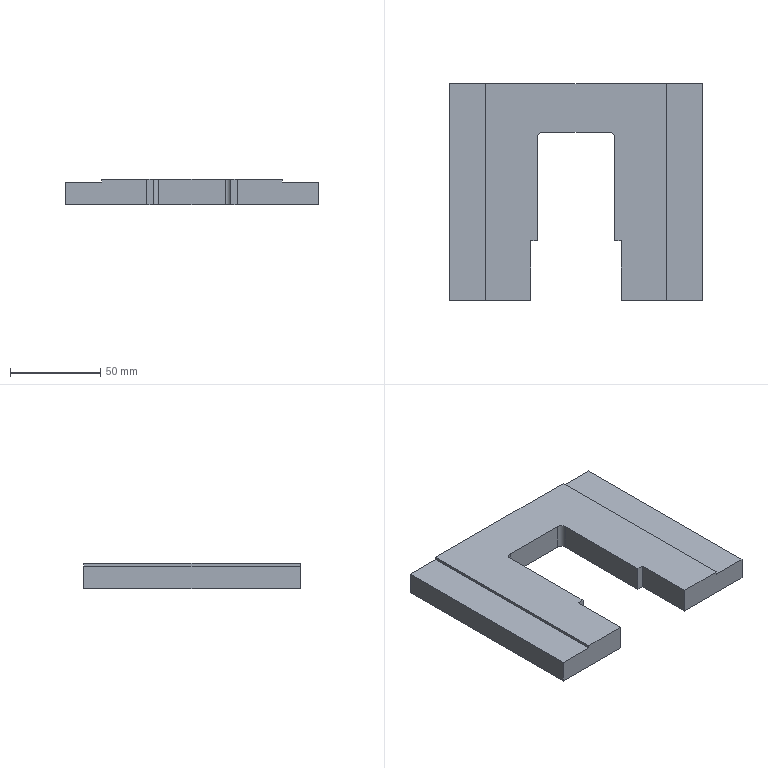Part | SolidWorks | features ICE 3, Extrusion 1, Fillet 1 | 1 solid | 20 faces | box 140 x 120 x 14 mm | volume 168834 mm3 | plane 18 | cylinder 2 | commonest cylinder face diameters 6 x2
STEP:
#1=CARTESIAN_POINT('',(-21.5,30.,14.));
#2=VERTEX_POINT('',#1);
#3=CARTESIAN_POINT('',(-21.5,-27.,14.));
#4=VERTEX_POINT('',#3);
#5=CARTESIAN_POINT('',(-21.5,-27.,14.));
#6=DIRECTION('',(0.,-1.,0.));
#7=VECTOR('',#6,1000.);
#8=LINE('',#5,#7);
#9=EDGE_CURVE('',#2,#4,#8,.T.);
#10=ORIENTED_EDGE('',*,*,#9,.F.);
#11=CARTESIAN_POINT('',(-18.5,33.,14.));
#12=VERTEX_POINT('',#11);
#13=CARTESIAN_POINT('',(-18.5,30.,14.));
#14=DIRECTION('',(0.,0.,-1.));
#15=DIRECTION('',(-1.,0.,0.));
#16=AXIS2_PLACEMENT_3D('',#13,#14,#15);
#17=CIRCLE('',#16,3.);
#18=EDGE_CURVE('',#2,#12,#17,.T.);
#19=ORIENTED_EDGE('',*,*,#18,.T.);
#20=CARTESIAN_POINT('',(18.5,33.,14.));
#21=VERTEX_POINT('',#20);
#22=CARTESIAN_POINT('',(-21.5,33.,14.));
#23=DIRECTION('',(-1.,0.,0.));
#24=VECTOR('',#23,1000.);
#25=LINE('',#22,#24);
#26=EDGE_CURVE('',#21,#12,#25,.T.);
#27=ORIENTED_EDGE('',*,*,#26,.F.);
#28=CARTESIAN_POINT('',(21.5,30.,14.));
#29=VERTEX_POINT('',#28);
#30=CARTESIAN_POINT('',(18.5,30.,14.));
#31=DIRECTION('',(0.,0.,-1.));
#32=DIRECTION('',(-1.,0.,0.));
#33=AXIS2_PLACEMENT_3D('',#30,#31,#32);
#34=CIRCLE('',#33,3.);
#35=EDGE_CURVE('',#21,#29,#34,.T.);
#36=ORIENTED_EDGE('',*,*,#35,.T.);
#37=CARTESIAN_POINT('',(21.5,-27.,14.));
#38=VERTEX_POINT('',#37);
#39=CARTESIAN_POINT('',(21.5,33.,14.));
#40=DIRECTION('',(0.,1.,0.));
#41=VECTOR('',#40,1000.);
#42=LINE('',#39,#41);
#43=EDGE_CURVE('',#38,#29,#42,.T.);
#44=ORIENTED_EDGE('',*,*,#43,.F.);
#45=CARTESIAN_POINT('',(25.,-27.,14.));
#46=VERTEX_POINT('',#45);
#47=CARTESIAN_POINT('',(25.,-27.,14.));
#48=DIRECTION('',(-1.,0.,0.));
#49=VECTOR('',#48,1000.);
#50=LINE('',#47,#49);
#51=EDGE_CURVE('',#46,#38,#50,.T.);
#52=ORIENTED_EDGE('',*,*,#51,.F.);
#53=CARTESIAN_POINT('',(25.,-60.,14.));
#54=VERTEX_POINT('',#53);
#55=CARTESIAN_POINT('',(25.,-60.,14.));
#56=DIRECTION('',(0.,1.,0.));
#57=VECTOR('',#56,1000.);
#58=LINE('',#55,#57);
#59=EDGE_CURVE('',#54,#46,#58,.T.);
#60=ORIENTED_EDGE('',*,*,#59,.F.);
#61=CARTESIAN_POINT('',(50.,-60.,14.));
#62=VERTEX_POINT('',#61);
#63=CARTESIAN_POINT('',(-70.,-60.,14.));
#64=DIRECTION('',(1.,0.,0.));
#65=VECTOR('',#64,1000.);
#66=LINE('',#63,#65);
#67=EDGE_CURVE('',#54,#62,#66,.T.);
#68=ORIENTED_EDGE('',*,*,#67,.T.);
#69=CARTESIAN_POINT('',(50.,60.,14.));
#70=VERTEX_POINT('',#69);
#71=CARTESIAN_POINT('',(50.,60.,14.));
#72=DIRECTION('',(0.,-1.,0.));
#73=VECTOR('',#72,1000.);
#74=LINE('',#71,#73);
#75=EDGE_CURVE('',#70,#62,#74,.T.);
#76=ORIENTED_EDGE('',*,*,#75,.F.);
#77=CARTESIAN_POINT('',(-50.,60.,14.));
#78=VERTEX_POINT('',#77);
#79=CARTESIAN_POINT('',(-70.,60.,14.));
#80=DIRECTION('',(-1.,0.,0.));
#81=VECTOR('',#80,1000.);
#82=LINE('',#79,#81);
#83=EDGE_CURVE('',#70,#78,#82,.T.);
#84=ORIENTED_EDGE('',*,*,#83,.T.);
#85=CARTESIAN_POINT('',(-50.,-60.,14.));
#86=VERTEX_POINT('',#85);
#87=CARTESIAN_POINT('',(-50.,60.,14.));
#88=DIRECTION('',(0.,1.,0.));
#89=VECTOR('',#88,1000.);
#90=LINE('',#87,#89);
#91=EDGE_CURVE('',#86,#78,#90,.T.);
#92=ORIENTED_EDGE('',*,*,#91,.F.);
#93=CARTESIAN_POINT('',(-25.,-60.,14.));
#94=VERTEX_POINT('',#93);
#95=CARTESIAN_POINT('',(-70.,-60.,14.));
#96=DIRECTION('',(1.,0.,0.));
#97=VECTOR('',#96,1000.);
#98=LINE('',#95,#97);
#99=EDGE_CURVE('',#86,#94,#98,.T.);
#100=ORIENTED_EDGE('',*,*,#99,.T.);
#101=CARTESIAN_POINT('',(-25.,-27.,14.));
#102=VERTEX_POINT('',#101);
#103=CARTESIAN_POINT('',(-25.,-27.,14.));
#104=DIRECTION('',(0.,-1.,0.));
#105=VECTOR('',#104,1000.);
#106=LINE('',#103,#105);
#107=EDGE_CURVE('',#102,#94,#106,.T.);
#108=ORIENTED_EDGE('',*,*,#107,.F.);
#109=CARTESIAN_POINT('',(25.,-27.,14.));
#110=DIRECTION('',(-1.,0.,0.));
#111=VECTOR('',#110,1000.);
#112=LINE('',#109,#111);
#113=EDGE_CURVE('',#4,#102,#112,.T.);
#114=ORIENTED_EDGE('',*,*,#113,.F.);
#115=EDGE_LOOP('',(#10,#19,#27,#36,#44,#52,#60,#68,#76,#84,#92,#100,#108,#114));
#116=FACE_OUTER_BOUND('',#115,.T.);
#117=CARTESIAN_POINT('',(0.,0.,14.));
#118=DIRECTION('',(0.,0.,-1.));
#119=DIRECTION('',(-1.,0.,0.));
#120=AXIS2_PLACEMENT_3D('',#117,#118,#119);
#121=PLANE('',#120);
#122=ADVANCED_FACE('',(#116),#121,.F.);
#123=CARTESIAN_POINT('',(21.5,-27.,0.));
#124=VERTEX_POINT('',#123);
#125=CARTESIAN_POINT('',(21.5,30.,0.));
#126=VERTEX_POINT('',#125);
#127=CARTESIAN_POINT('',(21.5,0.,0.));
#128=DIRECTION('',(0.,1.,0.));
#129=VECTOR('',#128,1000.);
#130=LINE('',#127,#129);
#131=EDGE_CURVE('',#124,#126,#130,.T.);
#132=ORIENTED_EDGE('',*,*,#131,.T.);
#133=CARTESIAN_POINT('',(18.5,33.,0.));
#134=VERTEX_POINT('',#133);
#135=CARTESIAN_POINT('',(18.5,30.,0.));
#136=DIRECTION('',(0.,0.,1.));
#137=DIRECTION('',(-1.,0.,0.));
#138=AXIS2_PLACEMENT_3D('',#135,#136,#137);
#139=CIRCLE('',#138,3.);
#140=EDGE_CURVE('',#126,#134,#139,.T.);
#141=ORIENTED_EDGE('',*,*,#140,.T.);
#142=CARTESIAN_POINT('',(-18.5,33.,0.));
#143=VERTEX_POINT('',#142);
#144=CARTESIAN_POINT('',(0.,33.,0.));
#145=DIRECTION('',(-1.,0.,0.));
#146=VECTOR('',#145,1000.);
#147=LINE('',#144,#146);
#148=EDGE_CURVE('',#134,#143,#147,.T.);
#149=ORIENTED_EDGE('',*,*,#148,.T.);
#150=CARTESIAN_POINT('',(-21.5,30.,0.));
#151=VERTEX_POINT('',#150);
#152=CARTESIAN_POINT('',(-18.5,30.,0.));
#153=DIRECTION('',(0.,0.,1.));
#154=DIRECTION('',(-1.,0.,0.));
#155=AXIS2_PLACEMENT_3D('',#152,#153,#154);
#156=CIRCLE('',#155,3.);
#157=EDGE_CURVE('',#143,#151,#156,.T.);
#158=ORIENTED_EDGE('',*,*,#157,.T.);
#159=CARTESIAN_POINT('',(-21.5,-27.,0.));
#160=VERTEX_POINT('',#159);
#161=CARTESIAN_POINT('',(-21.5,0.,0.));
#162=DIRECTION('',(0.,-1.,0.));
#163=VECTOR('',#162,1000.);
#164=LINE('',#161,#163);
#165=EDGE_CURVE('',#151,#160,#164,.T.);
#166=ORIENTED_EDGE('',*,*,#165,.T.);
#167=CARTESIAN_POINT('',(-25.,-27.,0.));
#168=VERTEX_POINT('',#167);
#169=CARTESIAN_POINT('',(25.,-27.,0.));
#170=DIRECTION('',(-1.,0.,0.));
#171=VECTOR('',#170,1000.);
#172=LINE('',#169,#171);
#173=EDGE_CURVE('',#160,#168,#172,.T.);
#174=ORIENTED_EDGE('',*,*,#173,.T.);
#175=CARTESIAN_POINT('',(-25.,-60.,0.));
#176=VERTEX_POINT('',#175);
#177=CARTESIAN_POINT('',(-25.,-27.,0.));
#178=DIRECTION('',(0.,-1.,0.));
#179=VECTOR('',#178,1000.);
#180=LINE('',#177,#179);
#181=EDGE_CURVE('',#168,#176,#180,.T.);
#182=ORIENTED_EDGE('',*,*,#181,.T.);
#183=CARTESIAN_POINT('',(-70.,-60.,0.));
#184=VERTEX_POINT('',#183);
#185=CARTESIAN_POINT('',(-70.,-60.,0.));
#186=DIRECTION('',(1.,0.,0.));
#187=VECTOR('',#186,1000.);
#188=LINE('',#185,#187);
#189=EDGE_CURVE('',#184,#176,#188,.T.);
#190=ORIENTED_EDGE('',*,*,#189,.F.);
#191=CARTESIAN_POINT('',(-70.,60.,0.));
#192=VERTEX_POINT('',#191);
#193=CARTESIAN_POINT('',(-70.,-60.,0.));
#194=DIRECTION('',(0.,-1.,0.));
#195=VECTOR('',#194,1000.);
#196=LINE('',#193,#195);
#197=EDGE_CURVE('',#192,#184,#196,.T.);
#198=ORIENTED_EDGE('',*,*,#197,.F.);
#199=CARTESIAN_POINT('',(70.,60.,0.));
#200=VERTEX_POINT('',#199);
#201=CARTESIAN_POINT('',(-70.,60.,0.));
#202=DIRECTION('',(-1.,0.,0.));
#203=VECTOR('',#202,1000.);
#204=LINE('',#201,#203);
#205=EDGE_CURVE('',#200,#192,#204,.T.);
#206=ORIENTED_EDGE('',*,*,#205,.F.);
#207=CARTESIAN_POINT('',(70.,-60.,0.));
#208=VERTEX_POINT('',#207);
#209=CARTESIAN_POINT('',(70.,-60.,0.));
#210=DIRECTION('',(0.,1.,0.));
#211=VECTOR('',#210,1000.);
#212=LINE('',#209,#211);
#213=EDGE_CURVE('',#208,#200,#212,.T.);
#214=ORIENTED_EDGE('',*,*,#213,.F.);
#215=CARTESIAN_POINT('',(25.,-60.,0.));
#216=VERTEX_POINT('',#215);
#217=CARTESIAN_POINT('',(-70.,-60.,0.));
#218=DIRECTION('',(1.,0.,0.));
#219=VECTOR('',#218,1000.);
#220=LINE('',#217,#219);
#221=EDGE_CURVE('',#216,#208,#220,.T.);
#222=ORIENTED_EDGE('',*,*,#221,.F.);
#223=CARTESIAN_POINT('',(25.,-27.,0.));
#224=VERTEX_POINT('',#223);
#225=CARTESIAN_POINT('',(25.,-60.,0.));
#226=DIRECTION('',(0.,1.,0.));
#227=VECTOR('',#226,1000.);
#228=LINE('',#225,#227);
#229=EDGE_CURVE('',#216,#224,#228,.T.);
#230=ORIENTED_EDGE('',*,*,#229,.T.);
#231=CARTESIAN_POINT('',(25.,-27.,0.));
#232=DIRECTION('',(-1.,0.,0.));
#233=VECTOR('',#232,1000.);
#234=LINE('',#231,#233);
#235=EDGE_CURVE('',#224,#124,#234,.T.);
#236=ORIENTED_EDGE('',*,*,#235,.T.);
#237=EDGE_LOOP('',(#132,#141,#149,#158,#166,#174,#182,#190,#198,#206,#214,#222,#230,#236));
#238=FACE_OUTER_BOUND('',#237,.T.);
#239=CARTESIAN_POINT('',(0.,0.,0.));
#240=DIRECTION('',(0.,0.,-1.));
#241=DIRECTION('',(-1.,0.,0.));
#242=AXIS2_PLACEMENT_3D('',#239,#240,#241);
#243=PLANE('',#242);
#244=ADVANCED_FACE('',(#238),#243,.T.);
#245=CARTESIAN_POINT('',(-21.5,-27.,-0.001));
#246=DIRECTION('',(0.,0.,-1.));
#247=VECTOR('',#246,1000.);
#248=LINE('',#245,#247);
#249=EDGE_CURVE('',#4,#160,#248,.T.);
#250=ORIENTED_EDGE('',*,*,#249,.F.);
#251=ORIENTED_EDGE('',*,*,#113,.T.);
#252=CARTESIAN_POINT('',(-25.,-27.,-0.001));
#253=DIRECTION('',(0.,0.,1.));
#254=VECTOR('',#253,1000.);
#255=LINE('',#252,#254);
#256=EDGE_CURVE('',#168,#102,#255,.T.);
#257=ORIENTED_EDGE('',*,*,#256,.F.);
#258=ORIENTED_EDGE('',*,*,#173,.F.);
#259=EDGE_LOOP('',(#250,#251,#257,#258));
#260=FACE_OUTER_BOUND('',#259,.T.);
#261=CARTESIAN_POINT('',(25.,-27.,-0.001));
#262=DIRECTION('',(0.,1.,0.));
#263=DIRECTION('',(-1.,0.,0.));
#264=AXIS2_PLACEMENT_3D('',#261,#262,#263);
#265=PLANE('',#264);
#266=ADVANCED_FACE('',(#260),#265,.F.);
#267=CARTESIAN_POINT('',(21.5,-27.,-0.001));
#268=DIRECTION('',(0.,0.,1.));
#269=VECTOR('',#268,1000.);
#270=LINE('',#267,#269);
#271=EDGE_CURVE('',#124,#38,#270,.T.);
#272=ORIENTED_EDGE('',*,*,#271,.F.);
#273=ORIENTED_EDGE('',*,*,#235,.F.);
#274=CARTESIAN_POINT('',(25.,-27.,-0.001));
#275=DIRECTION('',(0.,0.,1.));
#276=VECTOR('',#275,1000.);
#277=LINE('',#274,#276);
#278=EDGE_CURVE('',#224,#46,#277,.T.);
#279=ORIENTED_EDGE('',*,*,#278,.T.);
#280=ORIENTED_EDGE('',*,*,#51,.T.);
#281=EDGE_LOOP('',(#272,#273,#279,#280));
#282=FACE_OUTER_BOUND('',#281,.T.);
#283=CARTESIAN_POINT('',(25.,-27.,-0.001));
#284=DIRECTION('',(0.,1.,0.));
#285=DIRECTION('',(-1.,0.,0.));
#286=AXIS2_PLACEMENT_3D('',#283,#284,#285);
#287=PLANE('',#286);
#288=ADVANCED_FACE('',(#282),#287,.F.);
#289=ORIENTED_EDGE('',*,*,#189,.T.);
#290=CARTESIAN_POINT('',(-25.,-60.,-0.001));
#291=DIRECTION('',(0.,0.,1.));
#292=VECTOR('',#291,1000.);
#293=LINE('',#290,#292);
#294=EDGE_CURVE('',#176,#94,#293,.T.);
#295=ORIENTED_EDGE('',*,*,#294,.T.);
#296=ORIENTED_EDGE('',*,*,#99,.F.);
#297=CARTESIAN_POINT('',(-50.,-60.,12.5));
#298=VERTEX_POINT('',#297);
#299=CARTESIAN_POINT('',(-50.,-60.,12.5));
#300=DIRECTION('',(0.,0.,1.));
#301=VECTOR('',#300,1000.);
#302=LINE('',#299,#301);
#303=EDGE_CURVE('',#298,#86,#302,.T.);
#304=ORIENTED_EDGE('',*,*,#303,.F.);
#305=CARTESIAN_POINT('',(-70.,-60.,12.5));
#306=VERTEX_POINT('',#305);
#307=CARTESIAN_POINT('',(-70.,-60.,12.5));
#308=DIRECTION('',(1.,0.,0.));
#309=VECTOR('',#308,1000.);
#310=LINE('',#307,#309);
#311=EDGE_CURVE('',#306,#298,#310,.T.);
#312=ORIENTED_EDGE('',*,*,#311,.F.);
#313=CARTESIAN_POINT('',(-70.,-60.,14.));
#314=DIRECTION('',(0.,0.,-1.));
#315=VECTOR('',#314,1000.);
#316=LINE('',#313,#315);
#317=EDGE_CURVE('',#306,#184,#316,.T.);
#318=ORIENTED_EDGE('',*,*,#317,.T.);
#319=EDGE_LOOP('',(#289,#295,#296,#304,#312,#318));
#320=FACE_OUTER_BOUND('',#319,.T.);
#321=CARTESIAN_POINT('',(-70.,-60.,14.));
#322=DIRECTION('',(0.,1.,0.));
#323=DIRECTION('',(0.,0.,1.));
#324=AXIS2_PLACEMENT_3D('',#321,#322,#323);
#325=PLANE('',#324);
#326=ADVANCED_FACE('',(#320),#325,.F.);
#327=CARTESIAN_POINT('',(-70.,60.,12.5));
#328=VERTEX_POINT('',#327);
#329=CARTESIAN_POINT('',(-70.,60.,12.5));
#330=DIRECTION('',(0.,-1.,0.));
#331=VECTOR('',#330,1000.);
#332=LINE('',#329,#331);
#333=EDGE_CURVE('',#328,#306,#332,.T.);
#334=ORIENTED_EDGE('',*,*,#333,.F.);
#335=CARTESIAN_POINT('',(-70.,60.,14.));
#336=DIRECTION('',(0.,0.,-1.));
#337=VECTOR('',#336,1000.);
#338=LINE('',#335,#337);
#339=EDGE_CURVE('',#328,#192,#338,.T.);
#340=ORIENTED_EDGE('',*,*,#339,.T.);
#341=ORIENTED_EDGE('',*,*,#197,.T.);
#342=ORIENTED_EDGE('',*,*,#317,.F.);
#343=EDGE_LOOP('',(#334,#340,#341,#342));
#344=FACE_OUTER_BOUND('',#343,.T.);
#345=CARTESIAN_POINT('',(-70.,-60.,14.));
#346=DIRECTION('',(1.,0.,0.));
#347=DIRECTION('',(0.,0.,-1.));
#348=AXIS2_PLACEMENT_3D('',#345,#346,#347);
#349=PLANE('',#348);
#350=ADVANCED_FACE('',(#344),#349,.F.);
#351=CARTESIAN_POINT('',(70.,60.,12.5));
#352=VERTEX_POINT('',#351);
#353=CARTESIAN_POINT('',(70.,60.,14.));
#354=DIRECTION('',(0.,0.,-1.));
#355=VECTOR('',#354,1000.);
#356=LINE('',#353,#355);
#357=EDGE_CURVE('',#352,#200,#356,.T.);
#358=ORIENTED_EDGE('',*,*,#357,.F.);
#359=CARTESIAN_POINT('',(70.,-60.,12.5));
#360=VERTEX_POINT('',#359);
#361=CARTESIAN_POINT('',(70.,60.,12.5));
#362=DIRECTION('',(0.,1.,0.));
#363=VECTOR('',#362,1000.);
#364=LINE('',#361,#363);
#365=EDGE_CURVE('',#360,#352,#364,.T.);
#366=ORIENTED_EDGE('',*,*,#365,.F.);
#367=CARTESIAN_POINT('',(70.,-60.,14.));
#368=DIRECTION('',(0.,0.,-1.));
#369=VECTOR('',#368,1000.);
#370=LINE('',#367,#369);
#371=EDGE_CURVE('',#360,#208,#370,.T.);
#372=ORIENTED_EDGE('',*,*,#371,.T.);
#373=ORIENTED_EDGE('',*,*,#213,.T.);
#374=EDGE_LOOP('',(#358,#366,#372,#373));
#375=FACE_OUTER_BOUND('',#374,.T.);
#376=CARTESIAN_POINT('',(70.,-60.,14.));
#377=DIRECTION('',(-1.,0.,0.));
#378=DIRECTION('',(0.,0.,1.));
#379=AXIS2_PLACEMENT_3D('',#376,#377,#378);
#380=PLANE('',#379);
#381=ADVANCED_FACE('',(#375),#380,.F.);
#382=CARTESIAN_POINT('',(-50.,60.,12.5));
#383=VERTEX_POINT('',#382);
#384=CARTESIAN_POINT('',(-70.,60.,12.5));
#385=DIRECTION('',(-1.,0.,0.));
#386=VECTOR('',#385,1000.);
#387=LINE('',#384,#386);
#388=EDGE_CURVE('',#383,#328,#387,.T.);
#389=ORIENTED_EDGE('',*,*,#388,.F.);
#390=CARTESIAN_POINT('',(-50.,60.,12.5));
#391=DIRECTION('',(0.,0.,1.));
#392=VECTOR('',#391,1000.);
#393=LINE('',#390,#392);
#394=EDGE_CURVE('',#383,#78,#393,.T.);
#395=ORIENTED_EDGE('',*,*,#394,.T.);
#396=ORIENTED_EDGE('',*,*,#83,.F.);
#397=CARTESIAN_POINT('',(50.,60.,12.5));
#398=VERTEX_POINT('',#397);
#399=CARTESIAN_POINT('',(50.,60.,12.5));
#400=DIRECTION('',(0.,0.,1.));
#401=VECTOR('',#400,1000.);
#402=LINE('',#399,#401);
#403=EDGE_CURVE('',#398,#70,#402,.T.);
#404=ORIENTED_EDGE('',*,*,#403,.F.);
#405=CARTESIAN_POINT('',(70.,60.,12.5));
#406=DIRECTION('',(-1.,0.,0.));
#407=VECTOR('',#406,1000.);
#408=LINE('',#405,#407);
#409=EDGE_CURVE('',#352,#398,#408,.T.);
#410=ORIENTED_EDGE('',*,*,#409,.F.);
#411=ORIENTED_EDGE('',*,*,#357,.T.);
#412=ORIENTED_EDGE('',*,*,#205,.T.);
#413=ORIENTED_EDGE('',*,*,#339,.F.);
#414=EDGE_LOOP('',(#389,#395,#396,#404,#410,#411,#412,#413));
#415=FACE_OUTER_BOUND('',#414,.T.);
#416=CARTESIAN_POINT('',(-70.,60.,14.));
#417=DIRECTION('',(0.,-1.,0.));
#418=DIRECTION('',(0.,0.,-1.));
#419=AXIS2_PLACEMENT_3D('',#416,#417,#418);
#420=PLANE('',#419);
#421=ADVANCED_FACE('',(#415),#420,.F.);
#422=ORIENTED_EDGE('',*,*,#67,.F.);
#423=CARTESIAN_POINT('',(25.,-60.,-0.001));
#424=DIRECTION('',(0.,0.,1.));
#425=VECTOR('',#424,1000.);
#426=LINE('',#423,#425);
#427=EDGE_CURVE('',#216,#54,#426,.T.);
#428=ORIENTED_EDGE('',*,*,#427,.F.);
#429=ORIENTED_EDGE('',*,*,#221,.T.);
#430=ORIENTED_EDGE('',*,*,#371,.F.);
#431=CARTESIAN_POINT('',(50.,-60.,12.5));
#432=VERTEX_POINT('',#431);
#433=CARTESIAN_POINT('',(70.,-60.,12.5));
#434=DIRECTION('',(1.,0.,0.));
#435=VECTOR('',#434,1000.);
#436=LINE('',#433,#435);
#437=EDGE_CURVE('',#432,#360,#436,.T.);
#438=ORIENTED_EDGE('',*,*,#437,.F.);
#439=CARTESIAN_POINT('',(50.,-60.,12.5));
#440=DIRECTION('',(0.,0.,1.));
#441=VECTOR('',#440,1000.);
#442=LINE('',#439,#441);
#443=EDGE_CURVE('',#432,#62,#442,.T.);
#444=ORIENTED_EDGE('',*,*,#443,.T.);
#445=EDGE_LOOP('',(#422,#428,#429,#430,#438,#444));
#446=FACE_OUTER_BOUND('',#445,.T.);
#447=CARTESIAN_POINT('',(-70.,-60.,14.));
#448=DIRECTION('',(0.,1.,0.));
#449=DIRECTION('',(0.,0.,1.));
#450=AXIS2_PLACEMENT_3D('',#447,#448,#449);
#451=PLANE('',#450);
#452=ADVANCED_FACE('',(#446),#451,.F.);
#453=ORIENTED_EDGE('',*,*,#75,.T.);
#454=ORIENTED_EDGE('',*,*,#443,.F.);
#455=CARTESIAN_POINT('',(50.,60.,12.5));
#456=DIRECTION('',(0.,-1.,0.));
#457=VECTOR('',#456,1000.);
#458=LINE('',#455,#457);
#459=EDGE_CURVE('',#398,#432,#458,.T.);
#460=ORIENTED_EDGE('',*,*,#459,.F.);
#461=ORIENTED_EDGE('',*,*,#403,.T.);
#462=EDGE_LOOP('',(#453,#454,#460,#461));
#463=FACE_OUTER_BOUND('',#462,.T.);
#464=CARTESIAN_POINT('',(50.,60.,12.5));
#465=DIRECTION('',(-1.,0.,0.));
#466=DIRECTION('',(0.,-1.,0.));
#467=AXIS2_PLACEMENT_3D('',#464,#465,#466);
#468=PLANE('',#467);
#469=ADVANCED_FACE('',(#463),#468,.F.);
#470=ORIENTED_EDGE('',*,*,#365,.T.);
#471=ORIENTED_EDGE('',*,*,#409,.T.);
#472=ORIENTED_EDGE('',*,*,#459,.T.);
#473=ORIENTED_EDGE('',*,*,#437,.T.);
#474=EDGE_LOOP('',(#470,#471,#472,#473));
#475=FACE_OUTER_BOUND('',#474,.T.);
#476=CARTESIAN_POINT('',(0.,0.,12.5));
#477=DIRECTION('',(0.,0.,-1.));
#478=DIRECTION('',(-1.,0.,0.));
#479=AXIS2_PLACEMENT_3D('',#476,#477,#478);
#480=PLANE('',#479);
#481=ADVANCED_FACE('',(#475),#480,.F.);
#482=ORIENTED_EDGE('',*,*,#91,.T.);
#483=ORIENTED_EDGE('',*,*,#394,.F.);
#484=CARTESIAN_POINT('',(-50.,60.,12.5));
#485=DIRECTION('',(0.,1.,0.));
#486=VECTOR('',#485,1000.);
#487=LINE('',#484,#486);
#488=EDGE_CURVE('',#298,#383,#487,.T.);
#489=ORIENTED_EDGE('',*,*,#488,.F.);
#490=ORIENTED_EDGE('',*,*,#303,.T.);
#491=EDGE_LOOP('',(#482,#483,#489,#490));
#492=FACE_OUTER_BOUND('',#491,.T.);
#493=CARTESIAN_POINT('',(-50.,60.,12.5));
#494=DIRECTION('',(1.,0.,0.));
#495=DIRECTION('',(0.,1.,0.));
#496=AXIS2_PLACEMENT_3D('',#493,#494,#495);
#497=PLANE('',#496);
#498=ADVANCED_FACE('',(#492),#497,.F.);
#499=ORIENTED_EDGE('',*,*,#333,.T.);
#500=ORIENTED_EDGE('',*,*,#311,.T.);
#501=ORIENTED_EDGE('',*,*,#488,.T.);
#502=ORIENTED_EDGE('',*,*,#388,.T.);
#503=EDGE_LOOP('',(#499,#500,#501,#502));
#504=FACE_OUTER_BOUND('',#503,.T.);
#505=CARTESIAN_POINT('',(0.,0.,12.5));
#506=DIRECTION('',(0.,0.,1.));
#507=DIRECTION('',(1.,0.,0.));
#508=AXIS2_PLACEMENT_3D('',#505,#506,#507);
#509=PLANE('',#508);
#510=ADVANCED_FACE('',(#504),#509,.T.);
#511=ORIENTED_EDGE('',*,*,#256,.T.);
#512=ORIENTED_EDGE('',*,*,#107,.T.);
#513=ORIENTED_EDGE('',*,*,#294,.F.);
#514=ORIENTED_EDGE('',*,*,#181,.F.);
#515=EDGE_LOOP('',(#511,#512,#513,#514));
#516=FACE_OUTER_BOUND('',#515,.T.);
#517=CARTESIAN_POINT('',(-25.,-27.,-0.001));
#518=DIRECTION('',(-1.,0.,0.));
#519=DIRECTION('',(0.,-1.,0.));
#520=AXIS2_PLACEMENT_3D('',#517,#518,#519);
#521=PLANE('',#520);
#522=ADVANCED_FACE('',(#516),#521,.F.);
#523=ORIENTED_EDGE('',*,*,#427,.T.);
#524=ORIENTED_EDGE('',*,*,#59,.T.);
#525=ORIENTED_EDGE('',*,*,#278,.F.);
#526=ORIENTED_EDGE('',*,*,#229,.F.);
#527=EDGE_LOOP('',(#523,#524,#525,#526));
#528=FACE_OUTER_BOUND('',#527,.T.);
#529=CARTESIAN_POINT('',(25.,-60.,-0.001));
#530=DIRECTION('',(1.,0.,0.));
#531=DIRECTION('',(0.,1.,0.));
#532=AXIS2_PLACEMENT_3D('',#529,#530,#531);
#533=PLANE('',#532);
#534=ADVANCED_FACE('',(#528),#533,.F.);
#535=ORIENTED_EDGE('',*,*,#165,.F.);
#536=CARTESIAN_POINT('',(-21.5,30.,14.));
#537=DIRECTION('',(0.,0.,1.));
#538=VECTOR('',#537,1000.);
#539=LINE('',#536,#538);
#540=EDGE_CURVE('',#151,#2,#539,.T.);
#541=ORIENTED_EDGE('',*,*,#540,.T.);
#542=ORIENTED_EDGE('',*,*,#9,.T.);
#543=ORIENTED_EDGE('',*,*,#249,.T.);
#544=EDGE_LOOP('',(#535,#541,#542,#543));
#545=FACE_OUTER_BOUND('',#544,.T.);
#546=CARTESIAN_POINT('',(-21.5,-27.,-0.000012));
#547=DIRECTION('',(1.,0.,0.));
#548=DIRECTION('',(0.,1.,0.));
#549=AXIS2_PLACEMENT_3D('',#546,#547,#548);
#550=PLANE('',#549);
#551=ADVANCED_FACE('',(#545),#550,.T.);
#552=ORIENTED_EDGE('',*,*,#148,.F.);
#553=CARTESIAN_POINT('',(18.5,33.,14.));
#554=DIRECTION('',(0.,0.,1.));
#555=VECTOR('',#554,1000.);
#556=LINE('',#553,#555);
#557=EDGE_CURVE('',#134,#21,#556,.T.);
#558=ORIENTED_EDGE('',*,*,#557,.T.);
#559=ORIENTED_EDGE('',*,*,#26,.T.);
#560=CARTESIAN_POINT('',(-18.5,33.,0.));
#561=DIRECTION('',(0.,0.,-1.));
#562=VECTOR('',#561,1000.);
#563=LINE('',#560,#562);
#564=EDGE_CURVE('',#12,#143,#563,.T.);
#565=ORIENTED_EDGE('',*,*,#564,.T.);
#566=EDGE_LOOP('',(#552,#558,#559,#565));
#567=FACE_OUTER_BOUND('',#566,.T.);
#568=CARTESIAN_POINT('',(-21.5,33.,-0.000012));
#569=DIRECTION('',(0.,-1.,0.));
#570=DIRECTION('',(1.,0.,0.));
#571=AXIS2_PLACEMENT_3D('',#568,#569,#570);
#572=PLANE('',#571);
#573=ADVANCED_FACE('',(#567),#572,.T.);
#574=ORIENTED_EDGE('',*,*,#43,.T.);
#575=CARTESIAN_POINT('',(21.5,30.,0.));
#576=DIRECTION('',(0.,0.,-1.));
#577=VECTOR('',#576,1000.);
#578=LINE('',#575,#577);
#579=EDGE_CURVE('',#29,#126,#578,.T.);
#580=ORIENTED_EDGE('',*,*,#579,.T.);
#581=ORIENTED_EDGE('',*,*,#131,.F.);
#582=ORIENTED_EDGE('',*,*,#271,.T.);
#583=EDGE_LOOP('',(#574,#580,#581,#582));
#584=FACE_OUTER_BOUND('',#583,.T.);
#585=CARTESIAN_POINT('',(21.5,33.,-0.000012));
#586=DIRECTION('',(-1.,0.,0.));
#587=DIRECTION('',(0.,-1.,0.));
#588=AXIS2_PLACEMENT_3D('',#585,#586,#587);
#589=PLANE('',#588);
#590=ADVANCED_FACE('',(#584),#589,.T.);
#591=ORIENTED_EDGE('',*,*,#140,.F.);
#592=ORIENTED_EDGE('',*,*,#579,.F.);
#593=ORIENTED_EDGE('',*,*,#35,.F.);
#594=ORIENTED_EDGE('',*,*,#557,.F.);
#595=EDGE_LOOP('',(#591,#592,#593,#594));
#596=FACE_OUTER_BOUND('',#595,.T.);
#597=CARTESIAN_POINT('',(18.5,30.,-0.000012));
#598=DIRECTION('',(0.,0.,-1.));
#599=DIRECTION('',(-1.,0.,0.));
#600=AXIS2_PLACEMENT_3D('',#597,#598,#599);
#601=CYLINDRICAL_SURFACE('',#600,3.);
#602=ADVANCED_FACE('',(#596),#601,.F.);
#603=ORIENTED_EDGE('',*,*,#157,.F.);
#604=ORIENTED_EDGE('',*,*,#564,.F.);
#605=ORIENTED_EDGE('',*,*,#18,.F.);
#606=ORIENTED_EDGE('',*,*,#540,.F.);
#607=EDGE_LOOP('',(#603,#604,#605,#606));
#608=FACE_OUTER_BOUND('',#607,.T.);
#609=CARTESIAN_POINT('',(-18.5,30.,-0.000012));
#610=DIRECTION('',(0.,0.,-1.));
#611=DIRECTION('',(-1.,0.,0.));
#612=AXIS2_PLACEMENT_3D('',#609,#610,#611);
#613=CYLINDRICAL_SURFACE('',#612,3.);
#614=ADVANCED_FACE('',(#608),#613,.F.);
#615=CLOSED_SHELL('',(#122,#244,#266,#288,#326,#350,#381,#421,#452,#469,#481,#498,#510,#522,#534,#551,#573,#590,#602,#614));
#616=MANIFOLD_SOLID_BREP('',#615);
#617=CARTESIAN_POINT('',(0.,0.,0.));
#618=DIRECTION('',(0.,0.,1.));
#619=DIRECTION('',(1.,0.,0.));
#620=AXIS2_PLACEMENT_3D('',#617,#618,#619);
#621=(LENGTH_UNIT()NAMED_UNIT(*)SI_UNIT(.MILLI.,.METRE.));
#622=UNCERTAINTY_MEASURE_WITH_UNIT(LENGTH_MEASURE(0.00001),#621,'','');
#623=(NAMED_UNIT(*)PLANE_ANGLE_UNIT()SI_UNIT($,.RADIAN.));
#624=(NAMED_UNIT(*)SI_UNIT($,.STERADIAN.)SOLID_ANGLE_UNIT());
#625=(GEOMETRIC_REPRESENTATION_CONTEXT(3)GLOBAL_UNCERTAINTY_ASSIGNED_CONTEXT((#622))GLOBAL_UNIT_ASSIGNED_CONTEXT((#621,#623,#624))REPRESENTATION_CONTEXT('',''));
#626=ADVANCED_BREP_SHAPE_REPRESENTATION('',(#616,#620),#625);